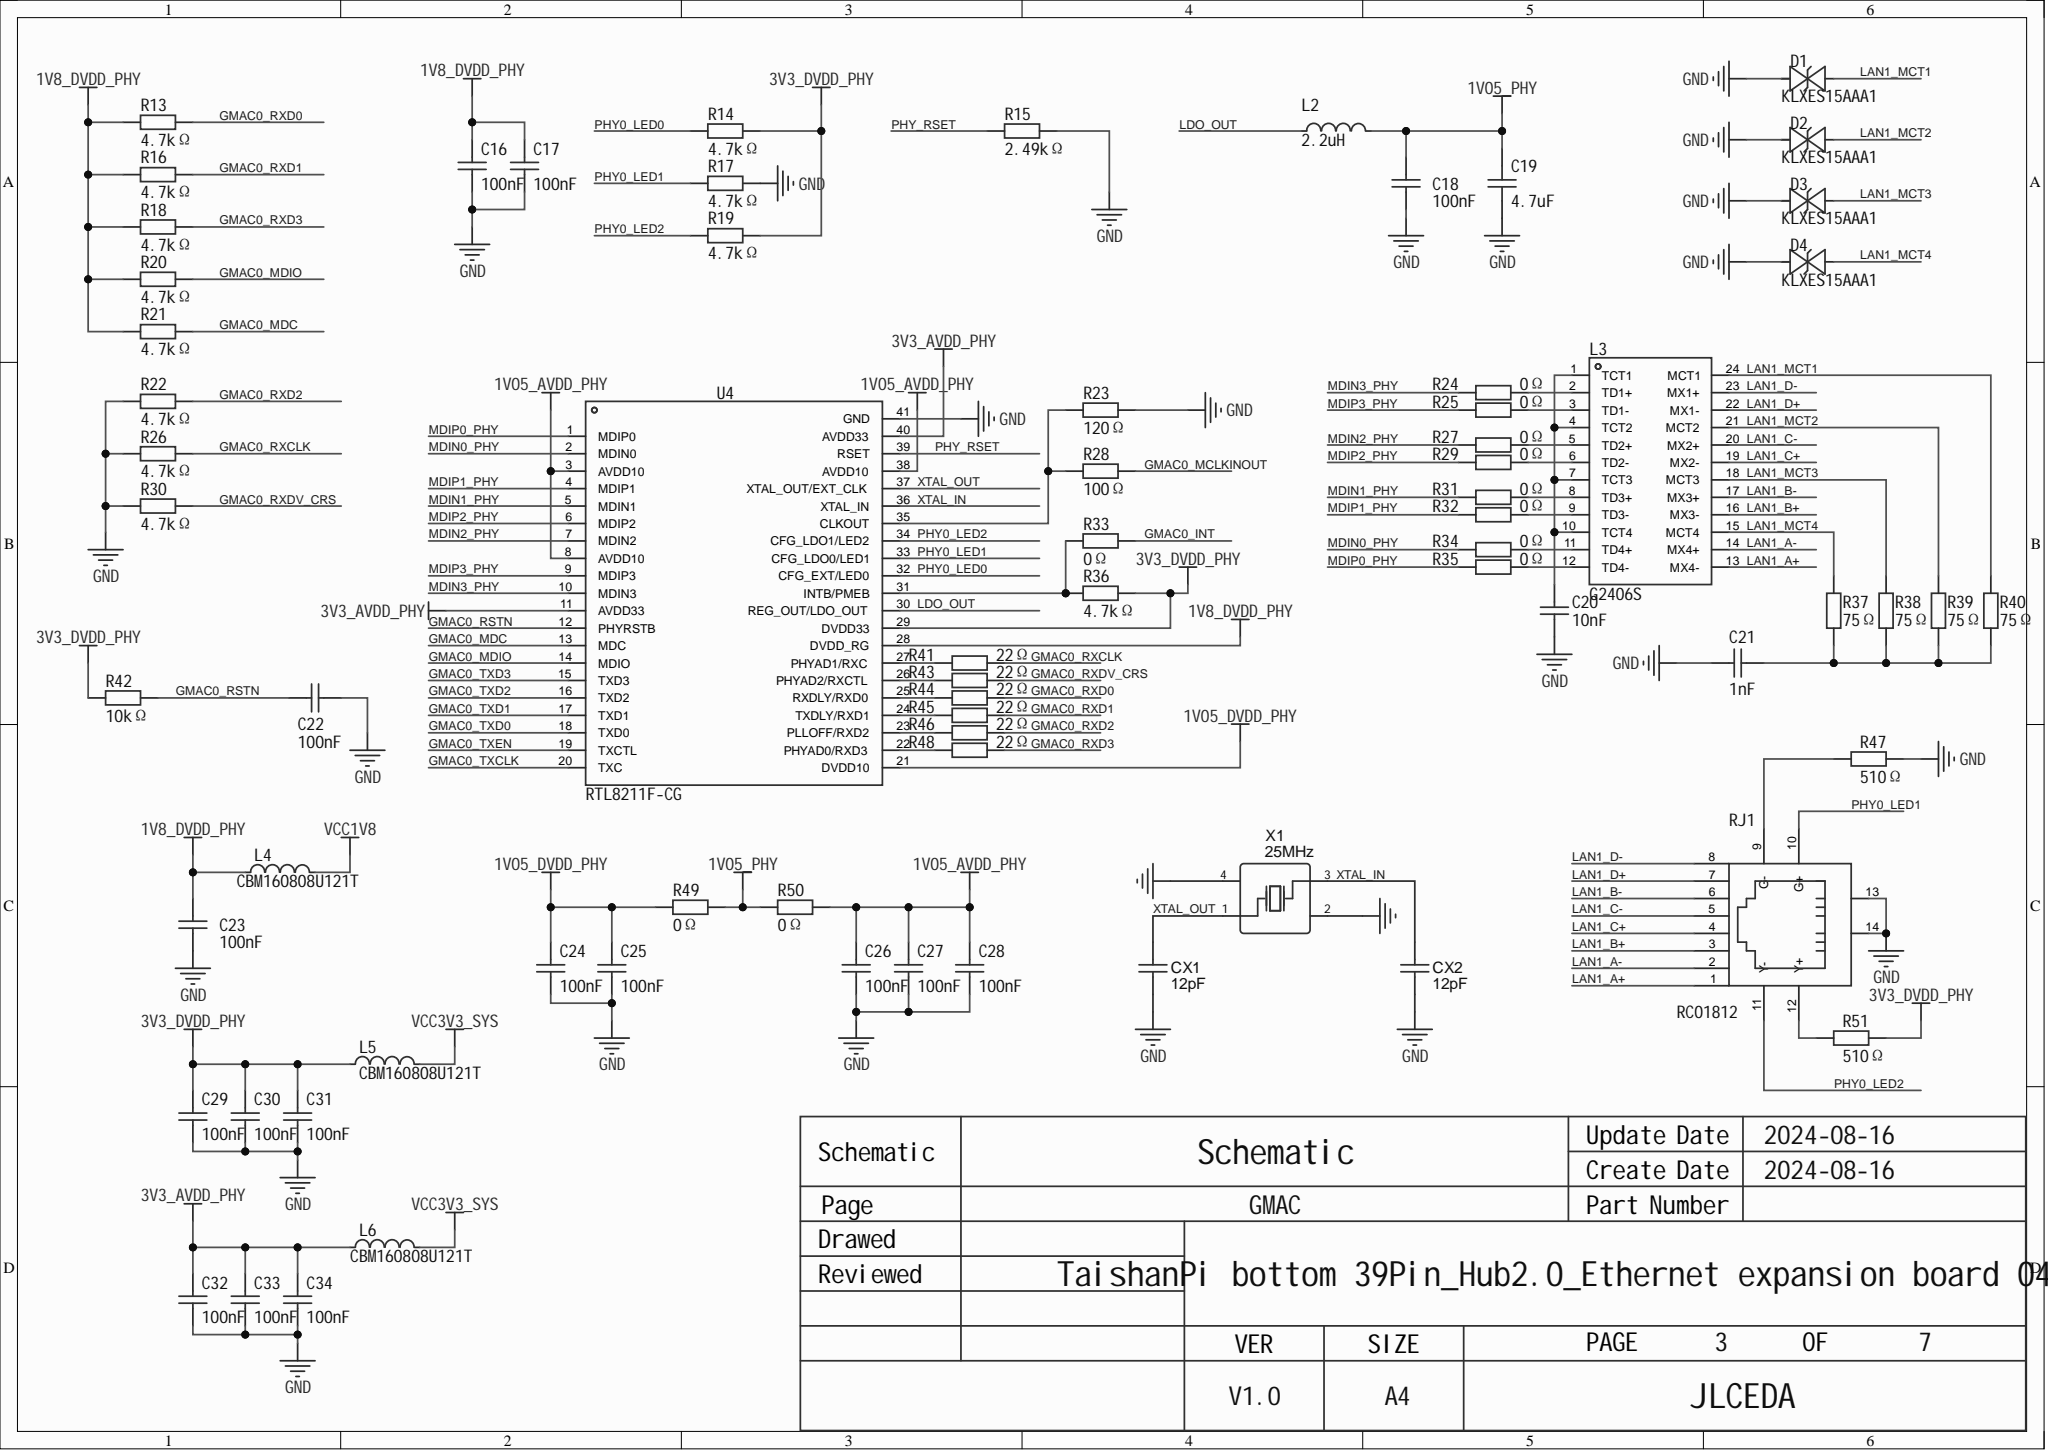Circuit board | Altium Designer | 209 parts | 149 nets | one sheet of the schematic
Parts on this sheet (reference | value | footprint):
C16 | 100nF | R0402
C17 | 100nF | R0402
C18 | 100nF | R0402
C19 | 4.7uF | R0402
C20 | 10nF | R1206
C21 | 1nF | R0402
C22 | 100nF | R0402
C23 | 100nF | R0402
C24 | 100nF | R0402
C25 | 100nF | R0402
C26 | 100nF | R0402
C27 | 100nF | R0402
C28 | 100nF | R0402
C29 | 100nF | R0402
C30 | 100nF | R0402
C31 | 100nF | R0402
C32 | 100nF | R0402
C33 | 100nF | R0402
C34 | 100nF | R0402
CX1 | 12pF | R0402
CX2 | 12pF | R0402
D1 | KLXES15AAA1 | D0402-BI
D2 | KLXES15AAA1 | D0402-BI
D3 | KLXES15AAA1 | D0402-BI
D4 | KLXES15AAA1 | D0402-BI
L2 | 2.2uH | IND-SMD_L2.5-W2.0_WPN252012H
L3 | G2406S | SMD-24_L15.1-W7.1-P1.00-LS10.0-BL
L4 | CBM160808U121T | L0603
L5 | CBM160808U121T | L0603
L6 | CBM160808U121T | L0603
R13 | 4.7kΩ | R0402
R14 | 4.7kΩ | R0402
R15 | 2.49kΩ | R0402
R16 | 4.7kΩ | R0402
R17 | 4.7kΩ | R0402
R18 | 4.7kΩ | R0402
R19 | 4.7kΩ | R0402
R20 | 4.7kΩ | R0402
R21 | 4.7kΩ | R0402
R22 | 4.7kΩ | R0402
R23 | 120Ω | R0402
R24 | 0Ω | R0402
R25 | 0Ω | R0402
R26 | 4.7kΩ | R0402
R27 | 0Ω | R0402
R28 | 100Ω | R0402
R29 | 0Ω | R0402
R30 | 4.7kΩ | R0402
R31 | 0Ω | R0402
R32 | 0Ω | R0402
R33 | 0Ω | R0402
R34 | 0Ω | R0402
R35 | 0Ω | R0402
R36 | 4.7kΩ | R0402
R37 | 75Ω | R0402
R38 | 75Ω | R0402
R39 | 75Ω | R0402
R40 | 75Ω | R0402
R41 | 22Ω | R0402
R42 | 10kΩ | R0402
R43 | 22Ω | R0402
R44 | 22Ω | R0402
R45 | 22Ω | R0402
R46 | 22Ω | R0402
R47 | 510Ω | R0402
R48 | 22Ω | R0402
R49 | 0Ω | R0402
R50 | 0Ω | R0402
R51 | 510Ω | R0402
RJ1 | RC01812 | RJ45-TH_RC01812
U4 | RTL8211F-CG | WQFN-40_L5.0-W5.0-P0.4-BL-EP
X1 | 25MHz | OSC-SMD_4P-L3.2-W2.5-BL
Nets of these parts (net: part-pin ...):
XTAL_OUT: CX1-2 X1-1 U4-37
XTAL_IN: CX2-2 X1-3 U4-36
VCC3V3_SYS: L5-2 L6-2
VCC1V8: L4-2
PHY_RSET: R15-1 U4-39
PHY0_LED2: R19-1 RJ1-11 U4-34
PHY0_LED1: R17-1 RJ1-10 U4-33
PHY0_LED0: R14-1 U4-32
NetR51_2: R51-2 RJ1-12
NetR48_1: R48-1 U4-22
NetR47_2: R47-2 RJ1-9
NetR46_1: R46-1 U4-23
NetR45_1: R45-1 U4-24
NetR44_1: R44-1 U4-25
NetR43_1: R43-1 U4-26
NetR41_1: R41-1 U4-27
NetR33_1: R33-1 R36-1 U4-31
NetR23_1: R23-1 R28-1 U4-35
NetL3_12: R35-2 L3-12
NetL3_11: R34-2 L3-11
NetL3_9: R32-2 L3-9
NetL3_8: R31-2 L3-8
NetL3_6: R29-2 L3-6
NetL3_5: R27-2 L3-5
NetL3_3: R25-2 L3-3
NetL3_2: R24-2 L3-2
NetC21_2: C21-2 R37-1 R38-1 R39-1 R40-1
NetC20_2: C20-2 L3-1 L3-4 L3-7 L3-10
MDIP3_PHY: R25-1 U4-9
MDIP2_PHY: R29-1 U4-6
MDIP1_PHY: R32-1 U4-4
MDIP0_PHY: R35-1 U4-1
MDIN3_PHY: R24-1 U4-10
MDIN2_PHY: R27-1 U4-7
MDIN1_PHY: R31-1 U4-5
MDIN0_PHY: R34-1 U4-2
LDO_OUT: L2-1 U4-30
LAN1_MCT4: D4-1 R37-2 L3-15
LAN1_MCT3: D3-1 R38-2 L3-18
LAN1_MCT2: D2-1 R39-2 L3-21
LAN1_MCT1: D1-1 R40-2 L3-24
LAN1_D-: RJ1-8 L3-23
LAN1_D+: RJ1-7 L3-22
LAN1_C-: RJ1-5 L3-20
LAN1_C+: RJ1-4 L3-19
LAN1_B-: RJ1-6 L3-17
LAN1_B+: RJ1-3 L3-16
LAN1_A-: RJ1-2 L3-14
LAN1_A+: RJ1-1 L3-13
GND: C16-1 C17-1 C18-1 C19-1 C20-1 C21-1 C22-1 C23-1 C24-1 C25-1 C26-1 C27-1 C28-1 C29-1 C30-1 C31-1 C32-1 C33-1 C34-1 CX1-1 CX2-1 D1-2 D2-2 D3-2 D4-2 R15-2 R17-2 R22-1 R23-2 R26-1 R30-1 R47-1 RJ1-13 RJ1-14 X1-2 X1-4 U4-41
GMAC0_TXEN: U4-19
GMAC0_TXD3: U4-15
GMAC0_TXD2: U4-16
GMAC0_TXD1: U4-17
GMAC0_TXD0: U4-18
GMAC0_TXCLK: U4-20
GMAC0_RXDV_CRS: R30-2 R43-2
GMAC0_RXD3: R18-2 R48-2
GMAC0_RXD2: R22-2 R46-2
GMAC0_RXD1: R16-2 R45-2
GMAC0_RXD0: R13-2 R44-2
GMAC0_RXCLK: R26-2 R41-2
GMAC0_RSTN: C22-2 R42-1 U4-12
GMAC0_MDIO: R20-2 U4-14
GMAC0_MDC: R21-2 U4-13
GMAC0_MCLKINOUT: R28-2
GMAC0_INT: R33-2
3V3_DVDD_PHY: C29-2 C30-2 C31-2 L5-1 R14-2 R19-2 R36-2 R42-2 R51-1 U4-29
3V3_AVDD_PHY: C32-2 C33-2 C34-2 L6-1 U4-11 U4-40
1V8_DVDD_PHY: C16-2 C17-2 C23-2 L4-1 R13-1 R16-1 R18-1 R20-1 R21-1 U4-28
1V05_PHY: C18-2 C19-2 L2-2 R49-2 R50-1
1V05_DVDD_PHY: C24-2 C25-2 R49-1 U4-21
1V05_AVDD_PHY: C26-2 C27-2 C28-2 R50-2 U4-3 U4-8 U4-38